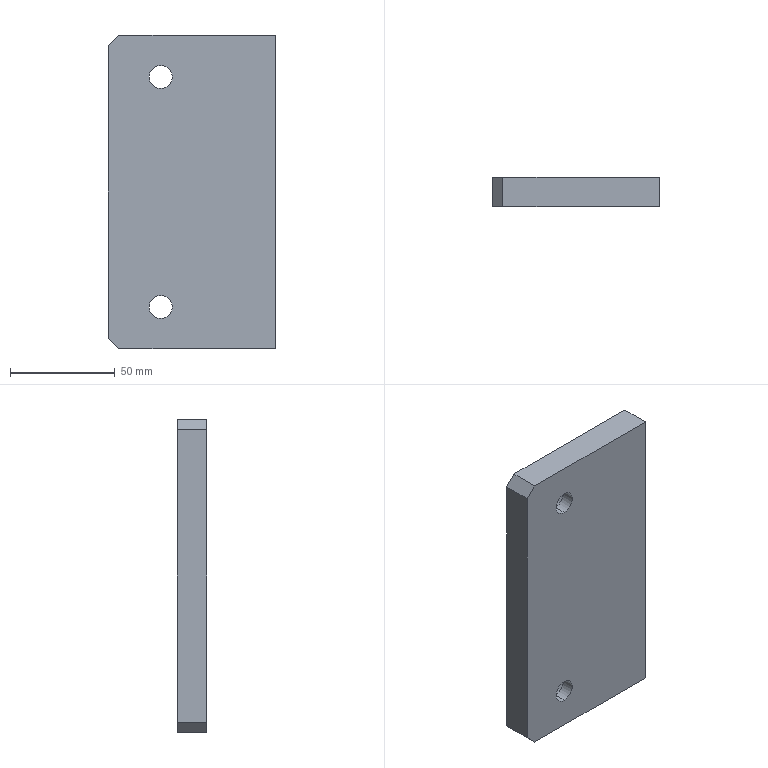Part | SolidWorks | features Chamfer 1, Extrusion 1, HoleWzd 1 | 1 solid | 18 faces | box 80 x 14 x 150 mm | volume 162438 mm3 | plane 10 | cylinder 8 | commonest cylinder face diameters 11 x4 18 x4
STEP:
#1=CARTESIAN_POINT('',(25.,6.,-139.));
#2=VERTEX_POINT('',#1);
#3=CARTESIAN_POINT('',(25.,6.,-121.));
#4=VERTEX_POINT('',#3);
#5=CARTESIAN_POINT('',(25.,6.,-130.));
#6=DIRECTION('',(0.,1.,0.));
#7=DIRECTION('',(0.,0.,1.));
#8=AXIS2_PLACEMENT_3D('',#5,#6,#7);
#9=CIRCLE('',#8,9.);
#10=EDGE_CURVE('',#2,#4,#9,.T.);
#11=ORIENTED_EDGE('',*,*,#10,.F.);
#12=CARTESIAN_POINT('',(25.,14.,-139.));
#13=VERTEX_POINT('',#12);
#14=CARTESIAN_POINT('',(25.,14.,-139.));
#15=DIRECTION('',(0.,1.,0.));
#16=VECTOR('',#15,1000.);
#17=LINE('',#14,#16);
#18=EDGE_CURVE('',#2,#13,#17,.T.);
#19=ORIENTED_EDGE('',*,*,#18,.T.);
#20=CARTESIAN_POINT('',(25.,14.,-121.));
#21=VERTEX_POINT('',#20);
#22=CARTESIAN_POINT('',(25.,14.,-130.));
#23=DIRECTION('',(0.,1.,0.));
#24=DIRECTION('',(0.,0.,1.));
#25=AXIS2_PLACEMENT_3D('',#22,#23,#24);
#26=CIRCLE('',#25,9.);
#27=EDGE_CURVE('',#13,#21,#26,.T.);
#28=ORIENTED_EDGE('',*,*,#27,.T.);
#29=CARTESIAN_POINT('',(25.,14.,-121.));
#30=DIRECTION('',(0.,1.,0.));
#31=VECTOR('',#30,1000.);
#32=LINE('',#29,#31);
#33=EDGE_CURVE('',#4,#21,#32,.T.);
#34=ORIENTED_EDGE('',*,*,#33,.F.);
#35=EDGE_LOOP('',(#11,#19,#28,#34));
#36=FACE_OUTER_BOUND('',#35,.T.);
#37=CARTESIAN_POINT('',(25.,14.,-130.));
#38=DIRECTION('',(0.,1.,0.));
#39=DIRECTION('',(0.,0.,1.));
#40=AXIS2_PLACEMENT_3D('',#37,#38,#39);
#41=CYLINDRICAL_SURFACE('',#40,9.);
#42=ADVANCED_FACE('',(#36),#41,.F.);
#43=CARTESIAN_POINT('',(25.,0.,-135.5));
#44=VERTEX_POINT('',#43);
#45=CARTESIAN_POINT('',(25.,0.,-124.5));
#46=VERTEX_POINT('',#45);
#47=CARTESIAN_POINT('',(25.,0.,-130.));
#48=DIRECTION('',(0.,1.,0.));
#49=DIRECTION('',(0.,0.,1.));
#50=AXIS2_PLACEMENT_3D('',#47,#48,#49);
#51=CIRCLE('',#50,5.5);
#52=EDGE_CURVE('',#44,#46,#51,.T.);
#53=ORIENTED_EDGE('',*,*,#52,.F.);
#54=CARTESIAN_POINT('',(25.,6.,-135.5));
#55=VERTEX_POINT('',#54);
#56=CARTESIAN_POINT('',(25.,14.,-135.5));
#57=DIRECTION('',(0.,1.,0.));
#58=VECTOR('',#57,1000.);
#59=LINE('',#56,#58);
#60=EDGE_CURVE('',#44,#55,#59,.T.);
#61=ORIENTED_EDGE('',*,*,#60,.T.);
#62=CARTESIAN_POINT('',(25.,6.,-124.5));
#63=VERTEX_POINT('',#62);
#64=CARTESIAN_POINT('',(25.,6.,-130.));
#65=DIRECTION('',(0.,1.,0.));
#66=DIRECTION('',(0.,0.,1.));
#67=AXIS2_PLACEMENT_3D('',#64,#65,#66);
#68=CIRCLE('',#67,5.5);
#69=EDGE_CURVE('',#55,#63,#68,.T.);
#70=ORIENTED_EDGE('',*,*,#69,.T.);
#71=CARTESIAN_POINT('',(25.,14.,-124.5));
#72=DIRECTION('',(0.,1.,0.));
#73=VECTOR('',#72,1000.);
#74=LINE('',#71,#73);
#75=EDGE_CURVE('',#46,#63,#74,.T.);
#76=ORIENTED_EDGE('',*,*,#75,.F.);
#77=EDGE_LOOP('',(#53,#61,#70,#76));
#78=FACE_OUTER_BOUND('',#77,.T.);
#79=CARTESIAN_POINT('',(25.,14.,-130.));
#80=DIRECTION('',(0.,1.,0.));
#81=DIRECTION('',(0.,0.,1.));
#82=AXIS2_PLACEMENT_3D('',#79,#80,#81);
#83=CYLINDRICAL_SURFACE('',#82,5.5);
#84=ADVANCED_FACE('',(#78),#83,.F.);
#85=CARTESIAN_POINT('',(25.,6.,-29.));
#86=VERTEX_POINT('',#85);
#87=CARTESIAN_POINT('',(25.,6.,-11.));
#88=VERTEX_POINT('',#87);
#89=CARTESIAN_POINT('',(25.,6.,-20.));
#90=DIRECTION('',(0.,1.,0.));
#91=DIRECTION('',(0.,0.,1.));
#92=AXIS2_PLACEMENT_3D('',#89,#90,#91);
#93=CIRCLE('',#92,9.);
#94=EDGE_CURVE('',#86,#88,#93,.T.);
#95=ORIENTED_EDGE('',*,*,#94,.F.);
#96=CARTESIAN_POINT('',(25.,14.,-29.));
#97=VERTEX_POINT('',#96);
#98=CARTESIAN_POINT('',(25.,14.,-29.));
#99=DIRECTION('',(0.,1.,0.));
#100=VECTOR('',#99,1000.);
#101=LINE('',#98,#100);
#102=EDGE_CURVE('',#86,#97,#101,.T.);
#103=ORIENTED_EDGE('',*,*,#102,.T.);
#104=CARTESIAN_POINT('',(25.,14.,-11.));
#105=VERTEX_POINT('',#104);
#106=CARTESIAN_POINT('',(25.,14.,-20.));
#107=DIRECTION('',(0.,1.,0.));
#108=DIRECTION('',(0.,0.,1.));
#109=AXIS2_PLACEMENT_3D('',#106,#107,#108);
#110=CIRCLE('',#109,9.);
#111=EDGE_CURVE('',#97,#105,#110,.T.);
#112=ORIENTED_EDGE('',*,*,#111,.T.);
#113=CARTESIAN_POINT('',(25.,14.,-11.));
#114=DIRECTION('',(0.,1.,0.));
#115=VECTOR('',#114,1000.);
#116=LINE('',#113,#115);
#117=EDGE_CURVE('',#88,#105,#116,.T.);
#118=ORIENTED_EDGE('',*,*,#117,.F.);
#119=EDGE_LOOP('',(#95,#103,#112,#118));
#120=FACE_OUTER_BOUND('',#119,.T.);
#121=CARTESIAN_POINT('',(25.,14.,-20.));
#122=DIRECTION('',(0.,1.,0.));
#123=DIRECTION('',(0.,0.,1.));
#124=AXIS2_PLACEMENT_3D('',#121,#122,#123);
#125=CYLINDRICAL_SURFACE('',#124,9.);
#126=ADVANCED_FACE('',(#120),#125,.F.);
#127=CARTESIAN_POINT('',(25.,0.,-25.5));
#128=VERTEX_POINT('',#127);
#129=CARTESIAN_POINT('',(25.,0.,-14.5));
#130=VERTEX_POINT('',#129);
#131=CARTESIAN_POINT('',(25.,0.,-20.));
#132=DIRECTION('',(0.,1.,0.));
#133=DIRECTION('',(0.,0.,1.));
#134=AXIS2_PLACEMENT_3D('',#131,#132,#133);
#135=CIRCLE('',#134,5.5);
#136=EDGE_CURVE('',#128,#130,#135,.T.);
#137=ORIENTED_EDGE('',*,*,#136,.F.);
#138=CARTESIAN_POINT('',(25.,6.,-25.5));
#139=VERTEX_POINT('',#138);
#140=CARTESIAN_POINT('',(25.,14.,-25.5));
#141=DIRECTION('',(0.,1.,0.));
#142=VECTOR('',#141,1000.);
#143=LINE('',#140,#142);
#144=EDGE_CURVE('',#128,#139,#143,.T.);
#145=ORIENTED_EDGE('',*,*,#144,.T.);
#146=CARTESIAN_POINT('',(25.,6.,-14.5));
#147=VERTEX_POINT('',#146);
#148=CARTESIAN_POINT('',(25.,6.,-20.));
#149=DIRECTION('',(0.,1.,0.));
#150=DIRECTION('',(0.,0.,1.));
#151=AXIS2_PLACEMENT_3D('',#148,#149,#150);
#152=CIRCLE('',#151,5.5);
#153=EDGE_CURVE('',#139,#147,#152,.T.);
#154=ORIENTED_EDGE('',*,*,#153,.T.);
#155=CARTESIAN_POINT('',(25.,14.,-14.5));
#156=DIRECTION('',(0.,1.,0.));
#157=VECTOR('',#156,1000.);
#158=LINE('',#155,#157);
#159=EDGE_CURVE('',#130,#147,#158,.T.);
#160=ORIENTED_EDGE('',*,*,#159,.F.);
#161=EDGE_LOOP('',(#137,#145,#154,#160));
#162=FACE_OUTER_BOUND('',#161,.T.);
#163=CARTESIAN_POINT('',(25.,14.,-20.));
#164=DIRECTION('',(0.,1.,0.));
#165=DIRECTION('',(0.,0.,1.));
#166=AXIS2_PLACEMENT_3D('',#163,#164,#165);
#167=CYLINDRICAL_SURFACE('',#166,5.5);
#168=ADVANCED_FACE('',(#162),#167,.F.);
#169=CARTESIAN_POINT('',(0.,0.,-145.));
#170=VERTEX_POINT('',#169);
#171=CARTESIAN_POINT('',(0.,0.,-5.));
#172=VERTEX_POINT('',#171);
#173=CARTESIAN_POINT('',(0.,0.,0.));
#174=DIRECTION('',(0.,0.,1.));
#175=VECTOR('',#174,1000.);
#176=LINE('',#173,#175);
#177=EDGE_CURVE('',#170,#172,#176,.T.);
#178=ORIENTED_EDGE('',*,*,#177,.T.);
#179=CARTESIAN_POINT('',(0.,14.,-5.));
#180=VERTEX_POINT('',#179);
#181=CARTESIAN_POINT('',(0.,14.,-5.));
#182=DIRECTION('',(0.,1.,0.));
#183=VECTOR('',#182,1000.);
#184=LINE('',#181,#183);
#185=EDGE_CURVE('',#172,#180,#184,.T.);
#186=ORIENTED_EDGE('',*,*,#185,.T.);
#187=CARTESIAN_POINT('',(0.,14.,-145.));
#188=VERTEX_POINT('',#187);
#189=CARTESIAN_POINT('',(0.,14.,0.));
#190=DIRECTION('',(0.,0.,1.));
#191=VECTOR('',#190,1000.);
#192=LINE('',#189,#191);
#193=EDGE_CURVE('',#188,#180,#192,.T.);
#194=ORIENTED_EDGE('',*,*,#193,.F.);
#195=CARTESIAN_POINT('',(0.,14.,-145.));
#196=DIRECTION('',(0.,-1.,0.));
#197=VECTOR('',#196,1000.);
#198=LINE('',#195,#197);
#199=EDGE_CURVE('',#188,#170,#198,.T.);
#200=ORIENTED_EDGE('',*,*,#199,.T.);
#201=EDGE_LOOP('',(#178,#186,#194,#200));
#202=FACE_OUTER_BOUND('',#201,.T.);
#203=CARTESIAN_POINT('',(0.,14.,0.));
#204=DIRECTION('',(1.,0.,0.));
#205=DIRECTION('',(0.,0.,-1.));
#206=AXIS2_PLACEMENT_3D('',#203,#204,#205);
#207=PLANE('',#206);
#208=ADVANCED_FACE('',(#202),#207,.F.);
#209=CARTESIAN_POINT('',(5.,14.,0.));
#210=VERTEX_POINT('',#209);
#211=CARTESIAN_POINT('',(80.,14.,0.));
#212=VERTEX_POINT('',#211);
#213=CARTESIAN_POINT('',(0.,14.,0.));
#214=DIRECTION('',(1.,0.,0.));
#215=VECTOR('',#214,1000.);
#216=LINE('',#213,#215);
#217=EDGE_CURVE('',#210,#212,#216,.T.);
#218=ORIENTED_EDGE('',*,*,#217,.F.);
#219=CARTESIAN_POINT('',(5.,0.,0.));
#220=VERTEX_POINT('',#219);
#221=CARTESIAN_POINT('',(5.,14.,0.));
#222=DIRECTION('',(0.,-1.,0.));
#223=VECTOR('',#222,1000.);
#224=LINE('',#221,#223);
#225=EDGE_CURVE('',#210,#220,#224,.T.);
#226=ORIENTED_EDGE('',*,*,#225,.T.);
#227=CARTESIAN_POINT('',(80.,0.,0.));
#228=VERTEX_POINT('',#227);
#229=CARTESIAN_POINT('',(0.,0.,0.));
#230=DIRECTION('',(1.,0.,0.));
#231=VECTOR('',#230,1000.);
#232=LINE('',#229,#231);
#233=EDGE_CURVE('',#220,#228,#232,.T.);
#234=ORIENTED_EDGE('',*,*,#233,.T.);
#235=CARTESIAN_POINT('',(80.,14.,0.));
#236=DIRECTION('',(0.,-1.,0.));
#237=VECTOR('',#236,1000.);
#238=LINE('',#235,#237);
#239=EDGE_CURVE('',#212,#228,#238,.T.);
#240=ORIENTED_EDGE('',*,*,#239,.F.);
#241=EDGE_LOOP('',(#218,#226,#234,#240));
#242=FACE_OUTER_BOUND('',#241,.T.);
#243=CARTESIAN_POINT('',(0.,14.,0.));
#244=DIRECTION('',(0.,0.,-1.));
#245=DIRECTION('',(-1.,0.,0.));
#246=AXIS2_PLACEMENT_3D('',#243,#244,#245);
#247=PLANE('',#246);
#248=ADVANCED_FACE('',(#242),#247,.F.);
#249=CARTESIAN_POINT('',(80.,0.,-150.));
#250=VERTEX_POINT('',#249);
#251=CARTESIAN_POINT('',(80.,0.,0.));
#252=DIRECTION('',(0.,0.,-1.));
#253=VECTOR('',#252,1000.);
#254=LINE('',#251,#253);
#255=EDGE_CURVE('',#228,#250,#254,.T.);
#256=ORIENTED_EDGE('',*,*,#255,.T.);
#257=CARTESIAN_POINT('',(80.,14.,-150.));
#258=VERTEX_POINT('',#257);
#259=CARTESIAN_POINT('',(80.,14.,-150.));
#260=DIRECTION('',(0.,-1.,0.));
#261=VECTOR('',#260,1000.);
#262=LINE('',#259,#261);
#263=EDGE_CURVE('',#258,#250,#262,.T.);
#264=ORIENTED_EDGE('',*,*,#263,.F.);
#265=CARTESIAN_POINT('',(80.,14.,0.));
#266=DIRECTION('',(0.,0.,-1.));
#267=VECTOR('',#266,1000.);
#268=LINE('',#265,#267);
#269=EDGE_CURVE('',#212,#258,#268,.T.);
#270=ORIENTED_EDGE('',*,*,#269,.F.);
#271=ORIENTED_EDGE('',*,*,#239,.T.);
#272=EDGE_LOOP('',(#256,#264,#270,#271));
#273=FACE_OUTER_BOUND('',#272,.T.);
#274=CARTESIAN_POINT('',(80.,14.,0.));
#275=DIRECTION('',(-1.,0.,0.));
#276=DIRECTION('',(0.,0.,1.));
#277=AXIS2_PLACEMENT_3D('',#274,#275,#276);
#278=PLANE('',#277);
#279=ADVANCED_FACE('',(#273),#278,.F.);
#280=CARTESIAN_POINT('',(5.,0.,-150.));
#281=VERTEX_POINT('',#280);
#282=CARTESIAN_POINT('',(0.,0.,-150.));
#283=DIRECTION('',(-1.,0.,0.));
#284=VECTOR('',#283,1000.);
#285=LINE('',#282,#284);
#286=EDGE_CURVE('',#250,#281,#285,.T.);
#287=ORIENTED_EDGE('',*,*,#286,.T.);
#288=CARTESIAN_POINT('',(5.,14.,-150.));
#289=VERTEX_POINT('',#288);
#290=CARTESIAN_POINT('',(5.,14.,-150.));
#291=DIRECTION('',(0.,1.,0.));
#292=VECTOR('',#291,1000.);
#293=LINE('',#290,#292);
#294=EDGE_CURVE('',#281,#289,#293,.T.);
#295=ORIENTED_EDGE('',*,*,#294,.T.);
#296=CARTESIAN_POINT('',(0.,14.,-150.));
#297=DIRECTION('',(-1.,0.,0.));
#298=VECTOR('',#297,1000.);
#299=LINE('',#296,#298);
#300=EDGE_CURVE('',#258,#289,#299,.T.);
#301=ORIENTED_EDGE('',*,*,#300,.F.);
#302=ORIENTED_EDGE('',*,*,#263,.T.);
#303=EDGE_LOOP('',(#287,#295,#301,#302));
#304=FACE_OUTER_BOUND('',#303,.T.);
#305=CARTESIAN_POINT('',(0.,14.,-150.));
#306=DIRECTION('',(0.,0.,1.));
#307=DIRECTION('',(1.,0.,0.));
#308=AXIS2_PLACEMENT_3D('',#305,#306,#307);
#309=PLANE('',#308);
#310=ADVANCED_FACE('',(#304),#309,.F.);
#311=CARTESIAN_POINT('',(25.,14.,-130.));
#312=DIRECTION('',(0.,1.,0.));
#313=DIRECTION('',(0.,0.,1.));
#314=AXIS2_PLACEMENT_3D('',#311,#312,#313);
#315=CIRCLE('',#314,9.);
#316=EDGE_CURVE('',#21,#13,#315,.T.);
#317=ORIENTED_EDGE('',*,*,#316,.F.);
#318=ORIENTED_EDGE('',*,*,#27,.F.);
#319=EDGE_LOOP('',(#317,#318));
#320=FACE_BOUND('',#319,.T.);
#321=CARTESIAN_POINT('',(25.,14.,-20.));
#322=DIRECTION('',(0.,1.,0.));
#323=DIRECTION('',(0.,0.,1.));
#324=AXIS2_PLACEMENT_3D('',#321,#322,#323);
#325=CIRCLE('',#324,9.);
#326=EDGE_CURVE('',#105,#97,#325,.T.);
#327=ORIENTED_EDGE('',*,*,#326,.F.);
#328=ORIENTED_EDGE('',*,*,#111,.F.);
#329=EDGE_LOOP('',(#327,#328));
#330=FACE_BOUND('',#329,.T.);
#331=ORIENTED_EDGE('',*,*,#193,.T.);
#332=CARTESIAN_POINT('',(5.,14.,0.));
#333=DIRECTION('',(0.7071,0.,0.7071));
#334=VECTOR('',#333,1000.);
#335=LINE('',#332,#334);
#336=EDGE_CURVE('',#180,#210,#335,.T.);
#337=ORIENTED_EDGE('',*,*,#336,.T.);
#338=ORIENTED_EDGE('',*,*,#217,.T.);
#339=ORIENTED_EDGE('',*,*,#269,.T.);
#340=ORIENTED_EDGE('',*,*,#300,.T.);
#341=CARTESIAN_POINT('',(0.,14.,-145.));
#342=DIRECTION('',(-0.7071,0.,0.7071));
#343=VECTOR('',#342,1000.);
#344=LINE('',#341,#343);
#345=EDGE_CURVE('',#289,#188,#344,.T.);
#346=ORIENTED_EDGE('',*,*,#345,.T.);
#347=EDGE_LOOP('',(#331,#337,#338,#339,#340,#346));
#348=FACE_OUTER_BOUND('',#347,.T.);
#349=CARTESIAN_POINT('',(0.,14.,0.));
#350=DIRECTION('',(0.,-1.,0.));
#351=DIRECTION('',(0.,0.,-1.));
#352=AXIS2_PLACEMENT_3D('',#349,#350,#351);
#353=PLANE('',#352);
#354=ADVANCED_FACE('',(#320,#330,#348),#353,.F.);
#355=CARTESIAN_POINT('',(25.,0.,-130.));
#356=DIRECTION('',(0.,1.,0.));
#357=DIRECTION('',(0.,0.,1.));
#358=AXIS2_PLACEMENT_3D('',#355,#356,#357);
#359=CIRCLE('',#358,5.5);
#360=EDGE_CURVE('',#46,#44,#359,.T.);
#361=ORIENTED_EDGE('',*,*,#360,.T.);
#362=ORIENTED_EDGE('',*,*,#52,.T.);
#363=EDGE_LOOP('',(#361,#362));
#364=FACE_BOUND('',#363,.T.);
#365=CARTESIAN_POINT('',(25.,0.,-20.));
#366=DIRECTION('',(0.,1.,0.));
#367=DIRECTION('',(0.,0.,1.));
#368=AXIS2_PLACEMENT_3D('',#365,#366,#367);
#369=CIRCLE('',#368,5.5);
#370=EDGE_CURVE('',#130,#128,#369,.T.);
#371=ORIENTED_EDGE('',*,*,#370,.T.);
#372=ORIENTED_EDGE('',*,*,#136,.T.);
#373=EDGE_LOOP('',(#371,#372));
#374=FACE_BOUND('',#373,.T.);
#375=ORIENTED_EDGE('',*,*,#233,.F.);
#376=CARTESIAN_POINT('',(2.5,0.,-2.5));
#377=DIRECTION('',(-0.7071,0.,-0.7071));
#378=VECTOR('',#377,1000.);
#379=LINE('',#376,#378);
#380=EDGE_CURVE('',#220,#172,#379,.T.);
#381=ORIENTED_EDGE('',*,*,#380,.T.);
#382=ORIENTED_EDGE('',*,*,#177,.F.);
#383=CARTESIAN_POINT('',(-72.5,0.,-72.5));
#384=DIRECTION('',(0.7071,0.,-0.7071));
#385=VECTOR('',#384,1000.);
#386=LINE('',#383,#385);
#387=EDGE_CURVE('',#170,#281,#386,.T.);
#388=ORIENTED_EDGE('',*,*,#387,.T.);
#389=ORIENTED_EDGE('',*,*,#286,.F.);
#390=ORIENTED_EDGE('',*,*,#255,.F.);
#391=EDGE_LOOP('',(#375,#381,#382,#388,#389,#390));
#392=FACE_OUTER_BOUND('',#391,.T.);
#393=CARTESIAN_POINT('',(0.,0.,0.));
#394=DIRECTION('',(0.,-1.,0.));
#395=DIRECTION('',(0.,0.,-1.));
#396=AXIS2_PLACEMENT_3D('',#393,#394,#395);
#397=PLANE('',#396);
#398=ADVANCED_FACE('',(#364,#374,#392),#397,.T.);
#399=ORIENTED_EDGE('',*,*,#144,.F.);
#400=ORIENTED_EDGE('',*,*,#370,.F.);
#401=ORIENTED_EDGE('',*,*,#159,.T.);
#402=CARTESIAN_POINT('',(25.,6.,-20.));
#403=DIRECTION('',(0.,1.,0.));
#404=DIRECTION('',(0.,0.,1.));
#405=AXIS2_PLACEMENT_3D('',#402,#403,#404);
#406=CIRCLE('',#405,5.5);
#407=EDGE_CURVE('',#147,#139,#406,.T.);
#408=ORIENTED_EDGE('',*,*,#407,.T.);
#409=EDGE_LOOP('',(#399,#400,#401,#408));
#410=FACE_OUTER_BOUND('',#409,.T.);
#411=CARTESIAN_POINT('',(25.,14.,-20.));
#412=DIRECTION('',(0.,1.,0.));
#413=DIRECTION('',(0.,0.,1.));
#414=AXIS2_PLACEMENT_3D('',#411,#412,#413);
#415=CYLINDRICAL_SURFACE('',#414,5.5);
#416=ADVANCED_FACE('',(#410),#415,.F.);
#417=ORIENTED_EDGE('',*,*,#407,.F.);
#418=ORIENTED_EDGE('',*,*,#153,.F.);
#419=EDGE_LOOP('',(#417,#418));
#420=FACE_BOUND('',#419,.T.);
#421=CARTESIAN_POINT('',(25.,6.,-20.));
#422=DIRECTION('',(0.,1.,0.));
#423=DIRECTION('',(0.,0.,1.));
#424=AXIS2_PLACEMENT_3D('',#421,#422,#423);
#425=CIRCLE('',#424,9.);
#426=EDGE_CURVE('',#88,#86,#425,.T.);
#427=ORIENTED_EDGE('',*,*,#426,.T.);
#428=ORIENTED_EDGE('',*,*,#94,.T.);
#429=EDGE_LOOP('',(#427,#428));
#430=FACE_OUTER_BOUND('',#429,.T.);
#431=CARTESIAN_POINT('',(30.5,6.,-20.));
#432=DIRECTION('',(0.,-1.,0.));
#433=DIRECTION('',(0.,0.,-1.));
#434=AXIS2_PLACEMENT_3D('',#431,#432,#433);
#435=PLANE('',#434);
#436=ADVANCED_FACE('',(#420,#430),#435,.F.);
#437=ORIENTED_EDGE('',*,*,#102,.F.);
#438=ORIENTED_EDGE('',*,*,#426,.F.);
#439=ORIENTED_EDGE('',*,*,#117,.T.);
#440=ORIENTED_EDGE('',*,*,#326,.T.);
#441=EDGE_LOOP('',(#437,#438,#439,#440));
#442=FACE_OUTER_BOUND('',#441,.T.);
#443=CARTESIAN_POINT('',(25.,14.,-20.));
#444=DIRECTION('',(0.,1.,0.));
#445=DIRECTION('',(0.,0.,1.));
#446=AXIS2_PLACEMENT_3D('',#443,#444,#445);
#447=CYLINDRICAL_SURFACE('',#446,9.);
#448=ADVANCED_FACE('',(#442),#447,.F.);
#449=ORIENTED_EDGE('',*,*,#60,.F.);
#450=ORIENTED_EDGE('',*,*,#360,.F.);
#451=ORIENTED_EDGE('',*,*,#75,.T.);
#452=CARTESIAN_POINT('',(25.,6.,-130.));
#453=DIRECTION('',(0.,1.,0.));
#454=DIRECTION('',(0.,0.,1.));
#455=AXIS2_PLACEMENT_3D('',#452,#453,#454);
#456=CIRCLE('',#455,5.5);
#457=EDGE_CURVE('',#63,#55,#456,.T.);
#458=ORIENTED_EDGE('',*,*,#457,.T.);
#459=EDGE_LOOP('',(#449,#450,#451,#458));
#460=FACE_OUTER_BOUND('',#459,.T.);
#461=CARTESIAN_POINT('',(25.,14.,-130.));
#462=DIRECTION('',(0.,1.,0.));
#463=DIRECTION('',(0.,0.,1.));
#464=AXIS2_PLACEMENT_3D('',#461,#462,#463);
#465=CYLINDRICAL_SURFACE('',#464,5.5);
#466=ADVANCED_FACE('',(#460),#465,.F.);
#467=ORIENTED_EDGE('',*,*,#457,.F.);
#468=ORIENTED_EDGE('',*,*,#69,.F.);
#469=EDGE_LOOP('',(#467,#468));
#470=FACE_BOUND('',#469,.T.);
#471=CARTESIAN_POINT('',(25.,6.,-130.));
#472=DIRECTION('',(0.,1.,0.));
#473=DIRECTION('',(0.,0.,1.));
#474=AXIS2_PLACEMENT_3D('',#471,#472,#473);
#475=CIRCLE('',#474,9.);
#476=EDGE_CURVE('',#4,#2,#475,.T.);
#477=ORIENTED_EDGE('',*,*,#476,.T.);
#478=ORIENTED_EDGE('',*,*,#10,.T.);
#479=EDGE_LOOP('',(#477,#478));
#480=FACE_OUTER_BOUND('',#479,.T.);
#481=CARTESIAN_POINT('',(30.5,6.,-130.));
#482=DIRECTION('',(0.,-1.,0.));
#483=DIRECTION('',(0.,0.,-1.));
#484=AXIS2_PLACEMENT_3D('',#481,#482,#483);
#485=PLANE('',#484);
#486=ADVANCED_FACE('',(#470,#480),#485,.F.);
#487=ORIENTED_EDGE('',*,*,#18,.F.);
#488=ORIENTED_EDGE('',*,*,#476,.F.);
#489=ORIENTED_EDGE('',*,*,#33,.T.);
#490=ORIENTED_EDGE('',*,*,#316,.T.);
#491=EDGE_LOOP('',(#487,#488,#489,#490));
#492=FACE_OUTER_BOUND('',#491,.T.);
#493=CARTESIAN_POINT('',(25.,14.,-130.));
#494=DIRECTION('',(0.,1.,0.));
#495=DIRECTION('',(0.,0.,1.));
#496=AXIS2_PLACEMENT_3D('',#493,#494,#495);
#497=CYLINDRICAL_SURFACE('',#496,9.);
#498=ADVANCED_FACE('',(#492),#497,.F.);
#499=ORIENTED_EDGE('',*,*,#336,.F.);
#500=ORIENTED_EDGE('',*,*,#185,.F.);
#501=ORIENTED_EDGE('',*,*,#380,.F.);
#502=ORIENTED_EDGE('',*,*,#225,.F.);
#503=EDGE_LOOP('',(#499,#500,#501,#502));
#504=FACE_OUTER_BOUND('',#503,.T.);
#505=CARTESIAN_POINT('',(5.,14.,0.));
#506=DIRECTION('',(0.7071,0.,-0.7071));
#507=DIRECTION('',(0.,-1.,0.));
#508=AXIS2_PLACEMENT_3D('',#505,#506,#507);
#509=PLANE('',#508);
#510=ADVANCED_FACE('',(#504),#509,.F.);
#511=ORIENTED_EDGE('',*,*,#345,.F.);
#512=ORIENTED_EDGE('',*,*,#294,.F.);
#513=ORIENTED_EDGE('',*,*,#387,.F.);
#514=ORIENTED_EDGE('',*,*,#199,.F.);
#515=EDGE_LOOP('',(#511,#512,#513,#514));
#516=FACE_OUTER_BOUND('',#515,.T.);
#517=CARTESIAN_POINT('',(0.,14.,-145.));
#518=DIRECTION('',(0.7071,0.,0.7071));
#519=DIRECTION('',(0.,-1.,0.));
#520=AXIS2_PLACEMENT_3D('',#517,#518,#519);
#521=PLANE('',#520);
#522=ADVANCED_FACE('',(#516),#521,.F.);
#523=CLOSED_SHELL('',(#42,#84,#126,#168,#208,#248,#279,#310,#354,#398,#416,#436,#448,#466,#486,#498,#510,#522));
#524=MANIFOLD_SOLID_BREP('',#523);
#525=CARTESIAN_POINT('',(0.,0.,0.));
#526=DIRECTION('',(0.,0.,1.));
#527=DIRECTION('',(1.,0.,0.));
#528=AXIS2_PLACEMENT_3D('',#525,#526,#527);
#529=(LENGTH_UNIT()NAMED_UNIT(*)SI_UNIT(.MILLI.,.METRE.));
#530=UNCERTAINTY_MEASURE_WITH_UNIT(LENGTH_MEASURE(0.00001),#529,'','');
#531=(NAMED_UNIT(*)PLANE_ANGLE_UNIT()SI_UNIT($,.RADIAN.));
#532=(NAMED_UNIT(*)SI_UNIT($,.STERADIAN.)SOLID_ANGLE_UNIT());
#533=(GEOMETRIC_REPRESENTATION_CONTEXT(3)GLOBAL_UNCERTAINTY_ASSIGNED_CONTEXT((#530))GLOBAL_UNIT_ASSIGNED_CONTEXT((#529,#531,#532))REPRESENTATION_CONTEXT('',''));
#534=ADVANCED_BREP_SHAPE_REPRESENTATION('',(#524,#528),#533);